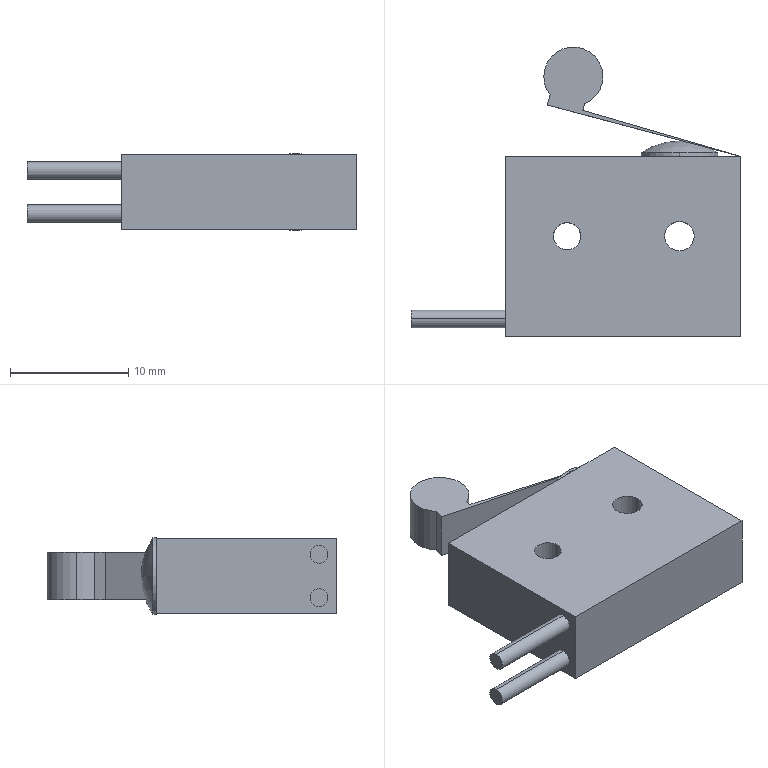Part | SolidWorks | features BaseBody 2 | 2 solids | 32 faces | box 27.9 x 24.5 x 6.5 mm | volume 2034 mm3 | plane 17 | cylinder 13 | sphere 2 | commonest cylinder face diameters 1.5 x4 5 x3 2.3 x2 2.5 x2 6.5 x2
STEP:
#1=CARTESIAN_POINT('',(-1.725,14.375,2.));
#2=VERTEX_POINT('',#1);
#3=CARTESIAN_POINT('',(-6.725,14.375,2.));
#4=VERTEX_POINT('',#3);
#5=CARTESIAN_POINT('',(-4.225,14.375,2.));
#6=DIRECTION('',(0.,0.,1.));
#7=DIRECTION('',(1.,0.,0.));
#8=AXIS2_PLACEMENT_3D('',#5,#6,#7);
#9=CIRCLE('',#8,2.5);
#10=EDGE_CURVE('',#2,#4,#9,.T.);
#11=ORIENTED_EDGE('',*,*,#10,.F.);
#12=CARTESIAN_POINT('',(-1.725,14.375,-2.));
#13=VERTEX_POINT('',#12);
#14=CARTESIAN_POINT('',(-1.725,14.375,2.));
#15=DIRECTION('',(0.,0.,-1.));
#16=VECTOR('',#15,1000.);
#17=LINE('',#14,#16);
#18=EDGE_CURVE('',#2,#13,#17,.T.);
#19=ORIENTED_EDGE('',*,*,#18,.T.);
#20=CARTESIAN_POINT('',(-6.725,14.375,-2.));
#21=VERTEX_POINT('',#20);
#22=CARTESIAN_POINT('',(-4.225,14.375,-2.));
#23=DIRECTION('',(0.,0.,1.));
#24=DIRECTION('',(1.,0.,0.));
#25=AXIS2_PLACEMENT_3D('',#22,#23,#24);
#26=CIRCLE('',#25,2.5);
#27=EDGE_CURVE('',#13,#21,#26,.T.);
#28=ORIENTED_EDGE('',*,*,#27,.T.);
#29=CARTESIAN_POINT('',(-6.725,14.375,2.));
#30=DIRECTION('',(0.,0.,-1.));
#31=VECTOR('',#30,1000.);
#32=LINE('',#29,#31);
#33=EDGE_CURVE('',#4,#21,#32,.T.);
#34=ORIENTED_EDGE('',*,*,#33,.F.);
#35=EDGE_LOOP('',(#11,#19,#28,#34));
#36=FACE_OUTER_BOUND('',#35,.T.);
#37=CARTESIAN_POINT('',(-4.225,14.375,2.));
#38=DIRECTION('',(0.,0.,-1.));
#39=DIRECTION('',(-1.,0.,0.));
#40=AXIS2_PLACEMENT_3D('',#37,#38,#39);
#41=CYLINDRICAL_SURFACE('',#40,2.5);
#42=ADVANCED_FACE('',(#36),#41,.T.);
#43=CARTESIAN_POINT('',(-6.187,12.826,2.));
#44=VERTEX_POINT('',#43);
#45=CARTESIAN_POINT('',(-4.225,14.375,2.));
#46=DIRECTION('',(0.,0.,1.));
#47=DIRECTION('',(1.,0.,0.));
#48=AXIS2_PLACEMENT_3D('',#45,#46,#47);
#49=CIRCLE('',#48,2.5);
#50=EDGE_CURVE('',#4,#44,#49,.T.);
#51=ORIENTED_EDGE('',*,*,#50,.F.);
#52=ORIENTED_EDGE('',*,*,#33,.T.);
#53=CARTESIAN_POINT('',(-6.187,12.826,-2.));
#54=VERTEX_POINT('',#53);
#55=CARTESIAN_POINT('',(-4.225,14.375,-2.));
#56=DIRECTION('',(0.,0.,1.));
#57=DIRECTION('',(1.,0.,0.));
#58=AXIS2_PLACEMENT_3D('',#55,#56,#57);
#59=CIRCLE('',#58,2.5);
#60=EDGE_CURVE('',#21,#54,#59,.T.);
#61=ORIENTED_EDGE('',*,*,#60,.T.);
#62=CARTESIAN_POINT('',(-6.187,12.826,2.));
#63=DIRECTION('',(0.,0.,-1.));
#64=VECTOR('',#63,1000.);
#65=LINE('',#62,#64);
#66=EDGE_CURVE('',#44,#54,#65,.T.);
#67=ORIENTED_EDGE('',*,*,#66,.F.);
#68=EDGE_LOOP('',(#51,#52,#61,#67));
#69=FACE_OUTER_BOUND('',#68,.T.);
#70=CARTESIAN_POINT('',(-4.225,14.375,2.));
#71=DIRECTION('',(0.,0.,-1.));
#72=DIRECTION('',(-1.,0.,0.));
#73=AXIS2_PLACEMENT_3D('',#70,#71,#72);
#74=CYLINDRICAL_SURFACE('',#73,2.5);
#75=ADVANCED_FACE('',(#69),#74,.T.);
#76=CARTESIAN_POINT('',(-3.429,11.526,-2.));
#77=VERTEX_POINT('',#76);
#78=CARTESIAN_POINT('',(9.95,7.625,-2.));
#79=VERTEX_POINT('',#78);
#80=CARTESIAN_POINT('',(-3.429,11.526,-2.));
#81=DIRECTION('',(0.96,-0.2799,0.));
#82=VECTOR('',#81,1000.);
#83=LINE('',#80,#82);
#84=EDGE_CURVE('',#77,#79,#83,.T.);
#85=ORIENTED_EDGE('',*,*,#84,.F.);
#86=CARTESIAN_POINT('',(-3.429,11.526,2.));
#87=VERTEX_POINT('',#86);
#88=CARTESIAN_POINT('',(-3.429,11.526,2.));
#89=DIRECTION('',(0.,0.,-1.));
#90=VECTOR('',#89,1000.);
#91=LINE('',#88,#90);
#92=EDGE_CURVE('',#87,#77,#91,.T.);
#93=ORIENTED_EDGE('',*,*,#92,.F.);
#94=CARTESIAN_POINT('',(9.95,7.625,2.));
#95=VERTEX_POINT('',#94);
#96=CARTESIAN_POINT('',(-3.429,11.526,2.));
#97=DIRECTION('',(0.96,-0.2799,0.));
#98=VECTOR('',#97,1000.);
#99=LINE('',#96,#98);
#100=EDGE_CURVE('',#87,#95,#99,.T.);
#101=ORIENTED_EDGE('',*,*,#100,.T.);
#102=CARTESIAN_POINT('',(9.95,7.625,2.));
#103=DIRECTION('',(0.,0.,-1.));
#104=VECTOR('',#103,1000.);
#105=LINE('',#102,#104);
#106=EDGE_CURVE('',#95,#79,#105,.T.);
#107=ORIENTED_EDGE('',*,*,#106,.T.);
#108=EDGE_LOOP('',(#85,#93,#101,#107));
#109=FACE_OUTER_BOUND('',#108,.T.);
#110=CARTESIAN_POINT('',(-3.429,11.526,2.));
#111=DIRECTION('',(0.2799,0.96,0.));
#112=DIRECTION('',(0.,0.,-1.));
#113=AXIS2_PLACEMENT_3D('',#110,#111,#112);
#114=PLANE('',#113);
#115=ADVANCED_FACE('',(#109),#114,.T.);
#116=CARTESIAN_POINT('',(-3.288,12.057,-2.));
#117=VERTEX_POINT('',#116);
#118=CARTESIAN_POINT('',(-3.288,12.057,-2.));
#119=DIRECTION('',(-0.2564,-0.9666,0.));
#120=VECTOR('',#119,1000.);
#121=LINE('',#118,#120);
#122=EDGE_CURVE('',#117,#77,#121,.T.);
#123=ORIENTED_EDGE('',*,*,#122,.F.);
#124=CARTESIAN_POINT('',(-3.288,12.057,2.));
#125=VERTEX_POINT('',#124);
#126=CARTESIAN_POINT('',(-3.288,12.057,2.));
#127=DIRECTION('',(0.,0.,-1.));
#128=VECTOR('',#127,1000.);
#129=LINE('',#126,#128);
#130=EDGE_CURVE('',#125,#117,#129,.T.);
#131=ORIENTED_EDGE('',*,*,#130,.F.);
#132=CARTESIAN_POINT('',(-3.288,12.057,2.));
#133=DIRECTION('',(-0.2564,-0.9666,0.));
#134=VECTOR('',#133,1000.);
#135=LINE('',#132,#134);
#136=EDGE_CURVE('',#125,#87,#135,.T.);
#137=ORIENTED_EDGE('',*,*,#136,.T.);
#138=ORIENTED_EDGE('',*,*,#92,.T.);
#139=EDGE_LOOP('',(#123,#131,#137,#138));
#140=FACE_OUTER_BOUND('',#139,.T.);
#141=CARTESIAN_POINT('',(-3.288,12.057,2.));
#142=DIRECTION('',(0.9666,-0.2564,0.));
#143=DIRECTION('',(0.,0.,-1.));
#144=AXIS2_PLACEMENT_3D('',#141,#142,#143);
#145=PLANE('',#144);
#146=ADVANCED_FACE('',(#140),#145,.T.);
#147=ORIENTED_EDGE('',*,*,#18,.F.);
#148=CARTESIAN_POINT('',(-4.225,14.375,2.));
#149=DIRECTION('',(0.,0.,1.));
#150=DIRECTION('',(1.,0.,0.));
#151=AXIS2_PLACEMENT_3D('',#148,#149,#150);
#152=CIRCLE('',#151,2.5);
#153=EDGE_CURVE('',#125,#2,#152,.T.);
#154=ORIENTED_EDGE('',*,*,#153,.F.);
#155=ORIENTED_EDGE('',*,*,#130,.T.);
#156=CARTESIAN_POINT('',(-4.225,14.375,-2.));
#157=DIRECTION('',(0.,0.,1.));
#158=DIRECTION('',(1.,0.,0.));
#159=AXIS2_PLACEMENT_3D('',#156,#157,#158);
#160=CIRCLE('',#159,2.5);
#161=EDGE_CURVE('',#117,#13,#160,.T.);
#162=ORIENTED_EDGE('',*,*,#161,.T.);
#163=EDGE_LOOP('',(#147,#154,#155,#162));
#164=FACE_OUTER_BOUND('',#163,.T.);
#165=CARTESIAN_POINT('',(-4.225,14.375,2.));
#166=DIRECTION('',(0.,0.,-1.));
#167=DIRECTION('',(-1.,0.,0.));
#168=AXIS2_PLACEMENT_3D('',#165,#166,#167);
#169=CYLINDRICAL_SURFACE('',#168,2.5);
#170=ADVANCED_FACE('',(#164),#169,.T.);
#171=CARTESIAN_POINT('',(-6.416,11.966,-2.));
#172=VERTEX_POINT('',#171);
#173=CARTESIAN_POINT('',(-6.416,11.966,-2.));
#174=DIRECTION('',(0.2564,0.9666,0.));
#175=VECTOR('',#174,1000.);
#176=LINE('',#173,#175);
#177=EDGE_CURVE('',#172,#54,#176,.T.);
#178=ORIENTED_EDGE('',*,*,#177,.F.);
#179=CARTESIAN_POINT('',(-6.416,11.966,2.));
#180=VERTEX_POINT('',#179);
#181=CARTESIAN_POINT('',(-6.416,11.966,2.));
#182=DIRECTION('',(0.,0.,-1.));
#183=VECTOR('',#182,1000.);
#184=LINE('',#181,#183);
#185=EDGE_CURVE('',#180,#172,#184,.T.);
#186=ORIENTED_EDGE('',*,*,#185,.F.);
#187=CARTESIAN_POINT('',(-6.416,11.966,2.));
#188=DIRECTION('',(0.2564,0.9666,0.));
#189=VECTOR('',#188,1000.);
#190=LINE('',#187,#189);
#191=EDGE_CURVE('',#180,#44,#190,.T.);
#192=ORIENTED_EDGE('',*,*,#191,.T.);
#193=ORIENTED_EDGE('',*,*,#66,.T.);
#194=EDGE_LOOP('',(#178,#186,#192,#193));
#195=FACE_OUTER_BOUND('',#194,.T.);
#196=CARTESIAN_POINT('',(-6.416,11.966,2.));
#197=DIRECTION('',(-0.9666,0.2564,0.));
#198=DIRECTION('',(0.,0.,1.));
#199=AXIS2_PLACEMENT_3D('',#196,#197,#198);
#200=PLANE('',#199);
#201=ADVANCED_FACE('',(#195),#200,.T.);
#202=CARTESIAN_POINT('',(9.95,7.625,-2.));
#203=DIRECTION('',(-0.9666,0.2564,0.));
#204=VECTOR('',#203,1000.);
#205=LINE('',#202,#204);
#206=EDGE_CURVE('',#79,#172,#205,.T.);
#207=ORIENTED_EDGE('',*,*,#206,.F.);
#208=ORIENTED_EDGE('',*,*,#106,.F.);
#209=CARTESIAN_POINT('',(9.95,7.625,2.));
#210=DIRECTION('',(-0.9666,0.2564,0.));
#211=VECTOR('',#210,1000.);
#212=LINE('',#209,#211);
#213=EDGE_CURVE('',#95,#180,#212,.T.);
#214=ORIENTED_EDGE('',*,*,#213,.T.);
#215=ORIENTED_EDGE('',*,*,#185,.T.);
#216=EDGE_LOOP('',(#207,#208,#214,#215));
#217=FACE_OUTER_BOUND('',#216,.T.);
#218=CARTESIAN_POINT('',(9.95,7.625,2.));
#219=DIRECTION('',(-0.2564,-0.9666,0.));
#220=DIRECTION('',(-0.9666,0.2564,0.));
#221=AXIS2_PLACEMENT_3D('',#218,#219,#220);
#222=PLANE('',#221);
#223=ADVANCED_FACE('',(#217),#222,.T.);
#224=ORIENTED_EDGE('',*,*,#100,.F.);
#225=ORIENTED_EDGE('',*,*,#136,.F.);
#226=ORIENTED_EDGE('',*,*,#153,.T.);
#227=ORIENTED_EDGE('',*,*,#10,.T.);
#228=ORIENTED_EDGE('',*,*,#50,.T.);
#229=ORIENTED_EDGE('',*,*,#191,.F.);
#230=ORIENTED_EDGE('',*,*,#213,.F.);
#231=EDGE_LOOP('',(#224,#225,#226,#227,#228,#229,#230));
#232=FACE_OUTER_BOUND('',#231,.T.);
#233=CARTESIAN_POINT('',(-4.225,14.375,2.));
#234=DIRECTION('',(0.,0.,1.));
#235=DIRECTION('',(1.,0.,0.));
#236=AXIS2_PLACEMENT_3D('',#233,#234,#235);
#237=PLANE('',#236);
#238=ADVANCED_FACE('',(#232),#237,.T.);
#239=ORIENTED_EDGE('',*,*,#84,.T.);
#240=ORIENTED_EDGE('',*,*,#206,.T.);
#241=ORIENTED_EDGE('',*,*,#177,.T.);
#242=ORIENTED_EDGE('',*,*,#60,.F.);
#243=ORIENTED_EDGE('',*,*,#27,.F.);
#244=ORIENTED_EDGE('',*,*,#161,.F.);
#245=ORIENTED_EDGE('',*,*,#122,.T.);
#246=EDGE_LOOP('',(#239,#240,#241,#242,#243,#244,#245));
#247=FACE_OUTER_BOUND('',#246,.T.);
#248=CARTESIAN_POINT('',(-4.225,14.375,-2.));
#249=DIRECTION('',(0.,0.,1.));
#250=DIRECTION('',(1.,0.,0.));
#251=AXIS2_PLACEMENT_3D('',#248,#249,#250);
#252=PLANE('',#251);
#253=ADVANCED_FACE('',(#247),#252,.F.);
#254=CLOSED_SHELL('',(#42,#75,#115,#146,#170,#201,#223,#238,#253));
#255=MANIFOLD_SOLID_BREP('',#254);
#256=CARTESIAN_POINT('',(4.75,7.925,-3.25));
#257=VERTEX_POINT('',#256);
#258=CARTESIAN_POINT('',(1.5,7.925,0.));
#259=VERTEX_POINT('',#258);
#260=CARTESIAN_POINT('',(4.75,7.925,0.));
#261=DIRECTION('',(0.,1.,0.));
#262=DIRECTION('',(0.,0.,1.));
#263=AXIS2_PLACEMENT_3D('',#260,#261,#262);
#264=CIRCLE('',#263,3.25);
#265=EDGE_CURVE('',#257,#259,#264,.T.);
#266=ORIENTED_EDGE('',*,*,#265,.T.);
#267=CARTESIAN_POINT('',(4.75,8.925,0.));
#268=VERTEX_POINT('',#267);
#269=CARTESIAN_POINT('',(4.75,3.144,0.));
#270=DIRECTION('',(0.,0.,-1.));
#271=DIRECTION('',(-1.,0.,0.));
#272=AXIS2_PLACEMENT_3D('',#269,#270,#271);
#273=CIRCLE('',#272,5.781);
#274=EDGE_CURVE('',#259,#268,#273,.T.);
#275=ORIENTED_EDGE('',*,*,#274,.T.);
#276=CARTESIAN_POINT('',(8.,7.925,0.));
#277=VERTEX_POINT('',#276);
#278=CARTESIAN_POINT('',(4.75,3.144,0.));
#279=DIRECTION('',(0.,0.,1.));
#280=DIRECTION('',(1.,0.,0.));
#281=AXIS2_PLACEMENT_3D('',#278,#279,#280);
#282=CIRCLE('',#281,5.781);
#283=EDGE_CURVE('',#277,#268,#282,.T.);
#284=ORIENTED_EDGE('',*,*,#283,.F.);
#285=CARTESIAN_POINT('',(4.75,7.925,0.));
#286=DIRECTION('',(0.,1.,0.));
#287=DIRECTION('',(0.,0.,1.));
#288=AXIS2_PLACEMENT_3D('',#285,#286,#287);
#289=CIRCLE('',#288,3.25);
#290=EDGE_CURVE('',#277,#257,#289,.T.);
#291=ORIENTED_EDGE('',*,*,#290,.T.);
#292=EDGE_LOOP('',(#266,#275,#284,#291));
#293=FACE_OUTER_BOUND('',#292,.T.);
#294=CARTESIAN_POINT('',(4.75,3.144,0.));
#295=DIRECTION('',(0.,0.,-1.));
#296=DIRECTION('',(1.,0.,0.));
#297=AXIS2_PLACEMENT_3D('',#294,#295,#296);
#298=SPHERICAL_SURFACE('',#297,5.781);
#299=ADVANCED_FACE('',(#293),#298,.T.);
#300=CARTESIAN_POINT('',(-17.95,-6.125,2.579));
#301=VERTEX_POINT('',#300);
#302=CARTESIAN_POINT('',(-17.95,-6.125,1.079));
#303=VERTEX_POINT('',#302);
#304=CARTESIAN_POINT('',(-17.95,-6.125,1.829));
#305=DIRECTION('',(-1.,0.,0.));
#306=DIRECTION('',(0.,0.,1.));
#307=AXIS2_PLACEMENT_3D('',#304,#305,#306);
#308=CIRCLE('',#307,0.75);
#309=EDGE_CURVE('',#301,#303,#308,.T.);
#310=ORIENTED_EDGE('',*,*,#309,.F.);
#311=CARTESIAN_POINT('',(-9.95,-6.125,2.579));
#312=VERTEX_POINT('',#311);
#313=CARTESIAN_POINT('',(-17.95,-6.125,2.579));
#314=DIRECTION('',(1.,0.,0.));
#315=VECTOR('',#314,1000.);
#316=LINE('',#313,#315);
#317=EDGE_CURVE('',#301,#312,#316,.T.);
#318=ORIENTED_EDGE('',*,*,#317,.T.);
#319=CARTESIAN_POINT('',(-9.95,-6.125,1.079));
#320=VERTEX_POINT('',#319);
#321=CARTESIAN_POINT('',(-9.95,-6.125,1.829));
#322=DIRECTION('',(-1.,0.,0.));
#323=DIRECTION('',(0.,0.,-1.));
#324=AXIS2_PLACEMENT_3D('',#321,#322,#323);
#325=CIRCLE('',#324,0.75);
#326=EDGE_CURVE('',#312,#320,#325,.T.);
#327=ORIENTED_EDGE('',*,*,#326,.T.);
#328=CARTESIAN_POINT('',(-17.95,-6.125,1.079));
#329=DIRECTION('',(1.,0.,0.));
#330=VECTOR('',#329,1000.);
#331=LINE('',#328,#330);
#332=EDGE_CURVE('',#303,#320,#331,.T.);
#333=ORIENTED_EDGE('',*,*,#332,.F.);
#334=EDGE_LOOP('',(#310,#318,#327,#333));
#335=FACE_OUTER_BOUND('',#334,.T.);
#336=CARTESIAN_POINT('',(-17.95,-6.125,1.829));
#337=DIRECTION('',(1.,0.,0.));
#338=DIRECTION('',(0.,0.,-1.));
#339=AXIS2_PLACEMENT_3D('',#336,#337,#338);
#340=CYLINDRICAL_SURFACE('',#339,0.75);
#341=ADVANCED_FACE('',(#335),#340,.T.);
#342=CARTESIAN_POINT('',(-17.95,-6.125,-1.079));
#343=VERTEX_POINT('',#342);
#344=CARTESIAN_POINT('',(-17.95,-6.125,-2.579));
#345=VERTEX_POINT('',#344);
#346=CARTESIAN_POINT('',(-17.95,-6.125,-1.829));
#347=DIRECTION('',(-1.,0.,0.));
#348=DIRECTION('',(0.,0.,1.));
#349=AXIS2_PLACEMENT_3D('',#346,#347,#348);
#350=CIRCLE('',#349,0.75);
#351=EDGE_CURVE('',#343,#345,#350,.T.);
#352=ORIENTED_EDGE('',*,*,#351,.F.);
#353=CARTESIAN_POINT('',(-9.95,-6.125,-1.079));
#354=VERTEX_POINT('',#353);
#355=CARTESIAN_POINT('',(-17.95,-6.125,-1.079));
#356=DIRECTION('',(1.,0.,0.));
#357=VECTOR('',#356,1000.);
#358=LINE('',#355,#357);
#359=EDGE_CURVE('',#343,#354,#358,.T.);
#360=ORIENTED_EDGE('',*,*,#359,.T.);
#361=CARTESIAN_POINT('',(-9.95,-6.125,-2.579));
#362=VERTEX_POINT('',#361);
#363=CARTESIAN_POINT('',(-9.95,-6.125,-1.829));
#364=DIRECTION('',(-1.,0.,0.));
#365=DIRECTION('',(0.,0.,-1.));
#366=AXIS2_PLACEMENT_3D('',#363,#364,#365);
#367=CIRCLE('',#366,0.75);
#368=EDGE_CURVE('',#354,#362,#367,.T.);
#369=ORIENTED_EDGE('',*,*,#368,.T.);
#370=CARTESIAN_POINT('',(-17.95,-6.125,-2.579));
#371=DIRECTION('',(1.,0.,0.));
#372=VECTOR('',#371,1000.);
#373=LINE('',#370,#372);
#374=EDGE_CURVE('',#345,#362,#373,.T.);
#375=ORIENTED_EDGE('',*,*,#374,.F.);
#376=EDGE_LOOP('',(#352,#360,#369,#375));
#377=FACE_OUTER_BOUND('',#376,.T.);
#378=CARTESIAN_POINT('',(-17.95,-6.125,-1.829));
#379=DIRECTION('',(1.,0.,0.));
#380=DIRECTION('',(0.,0.,-1.));
#381=AXIS2_PLACEMENT_3D('',#378,#379,#380);
#382=CYLINDRICAL_SURFACE('',#381,0.75);
#383=ADVANCED_FACE('',(#377),#382,.T.);
#384=CARTESIAN_POINT('',(4.75,7.925,3.25));
#385=VERTEX_POINT('',#384);
#386=CARTESIAN_POINT('',(4.75,7.925,0.));
#387=DIRECTION('',(0.,1.,0.));
#388=DIRECTION('',(0.,0.,1.));
#389=AXIS2_PLACEMENT_3D('',#386,#387,#388);
#390=CIRCLE('',#389,3.25);
#391=EDGE_CURVE('',#385,#277,#390,.T.);
#392=ORIENTED_EDGE('',*,*,#391,.F.);
#393=CARTESIAN_POINT('',(4.75,7.625,3.25));
#394=VERTEX_POINT('',#393);
#395=CARTESIAN_POINT('',(4.75,7.925,3.25));
#396=DIRECTION('',(0.,-1.,0.));
#397=VECTOR('',#396,1000.);
#398=LINE('',#395,#397);
#399=EDGE_CURVE('',#385,#394,#398,.T.);
#400=ORIENTED_EDGE('',*,*,#399,.T.);
#401=CARTESIAN_POINT('',(5.318,7.625,3.2));
#402=VERTEX_POINT('',#401);
#403=CARTESIAN_POINT('',(4.75,7.625,0.));
#404=DIRECTION('',(0.,1.,0.));
#405=DIRECTION('',(0.,0.,1.));
#406=AXIS2_PLACEMENT_3D('',#403,#404,#405);
#407=CIRCLE('',#406,3.25);
#408=EDGE_CURVE('',#394,#402,#407,.T.);
#409=ORIENTED_EDGE('',*,*,#408,.T.);
#410=CARTESIAN_POINT('',(5.318,7.625,-3.2));
#411=VERTEX_POINT('',#410);
#412=CARTESIAN_POINT('',(4.75,7.625,0.));
#413=DIRECTION('',(0.,1.,0.));
#414=DIRECTION('',(0.,0.,1.));
#415=AXIS2_PLACEMENT_3D('',#412,#413,#414);
#416=CIRCLE('',#415,3.25);
#417=EDGE_CURVE('',#402,#411,#416,.T.);
#418=ORIENTED_EDGE('',*,*,#417,.T.);
#419=CARTESIAN_POINT('',(4.75,7.625,-3.25));
#420=VERTEX_POINT('',#419);
#421=CARTESIAN_POINT('',(4.75,7.625,0.));
#422=DIRECTION('',(0.,1.,0.));
#423=DIRECTION('',(0.,0.,1.));
#424=AXIS2_PLACEMENT_3D('',#421,#422,#423);
#425=CIRCLE('',#424,3.25);
#426=EDGE_CURVE('',#411,#420,#425,.T.);
#427=ORIENTED_EDGE('',*,*,#426,.T.);
#428=CARTESIAN_POINT('',(4.75,7.925,-3.25));
#429=DIRECTION('',(0.,-1.,0.));
#430=VECTOR('',#429,1000.);
#431=LINE('',#428,#430);
#432=EDGE_CURVE('',#257,#420,#431,.T.);
#433=ORIENTED_EDGE('',*,*,#432,.F.);
#434=ORIENTED_EDGE('',*,*,#290,.F.);
#435=EDGE_LOOP('',(#392,#400,#409,#418,#427,#433,#434));
#436=FACE_OUTER_BOUND('',#435,.T.);
#437=CARTESIAN_POINT('',(4.75,7.925,0.));
#438=DIRECTION('',(0.,-1.,0.));
#439=DIRECTION('',(0.,0.,-1.));
#440=AXIS2_PLACEMENT_3D('',#437,#438,#439);
#441=CYLINDRICAL_SURFACE('',#440,3.25);
#442=ADVANCED_FACE('',(#436),#441,.T.);
#443=CARTESIAN_POINT('',(3.5,0.875,3.2));
#444=VERTEX_POINT('',#443);
#445=CARTESIAN_POINT('',(6.,0.875,3.2));
#446=VERTEX_POINT('',#445);
#447=CARTESIAN_POINT('',(4.75,0.875,3.2));
#448=DIRECTION('',(0.,0.,1.));
#449=DIRECTION('',(1.,0.,0.));
#450=AXIS2_PLACEMENT_3D('',#447,#448,#449);
#451=CIRCLE('',#450,1.25);
#452=EDGE_CURVE('',#444,#446,#451,.T.);
#453=ORIENTED_EDGE('',*,*,#452,.T.);
#454=CARTESIAN_POINT('',(6.,0.875,-3.2));
#455=VERTEX_POINT('',#454);
#456=CARTESIAN_POINT('',(6.,0.875,3.2));
#457=DIRECTION('',(0.,0.,-1.));
#458=VECTOR('',#457,1000.);
#459=LINE('',#456,#458);
#460=EDGE_CURVE('',#446,#455,#459,.T.);
#461=ORIENTED_EDGE('',*,*,#460,.T.);
#462=CARTESIAN_POINT('',(3.5,0.875,-3.2));
#463=VERTEX_POINT('',#462);
#464=CARTESIAN_POINT('',(4.75,0.875,-3.2));
#465=DIRECTION('',(0.,0.,1.));
#466=DIRECTION('',(1.,0.,0.));
#467=AXIS2_PLACEMENT_3D('',#464,#465,#466);
#468=CIRCLE('',#467,1.25);
#469=EDGE_CURVE('',#463,#455,#468,.T.);
#470=ORIENTED_EDGE('',*,*,#469,.F.);
#471=CARTESIAN_POINT('',(3.5,0.875,3.2));
#472=DIRECTION('',(0.,0.,-1.));
#473=VECTOR('',#472,1000.);
#474=LINE('',#471,#473);
#475=EDGE_CURVE('',#444,#463,#474,.T.);
#476=ORIENTED_EDGE('',*,*,#475,.F.);
#477=EDGE_LOOP('',(#453,#461,#470,#476));
#478=FACE_OUTER_BOUND('',#477,.T.);
#479=CARTESIAN_POINT('',(4.75,0.875,3.2));
#480=DIRECTION('',(0.,0.,-1.));
#481=DIRECTION('',(-1.,0.,0.));
#482=AXIS2_PLACEMENT_3D('',#479,#480,#481);
#483=CYLINDRICAL_SURFACE('',#482,1.25);
#484=ADVANCED_FACE('',(#478),#483,.F.);
#485=CARTESIAN_POINT('',(-5.9,0.875,3.2));
#486=VERTEX_POINT('',#485);
#487=CARTESIAN_POINT('',(-3.6,0.875,3.2));
#488=VERTEX_POINT('',#487);
#489=CARTESIAN_POINT('',(-4.75,0.875,3.2));
#490=DIRECTION('',(0.,0.,1.));
#491=DIRECTION('',(1.,0.,0.));
#492=AXIS2_PLACEMENT_3D('',#489,#490,#491);
#493=CIRCLE('',#492,1.15);
#494=EDGE_CURVE('',#486,#488,#493,.T.);
#495=ORIENTED_EDGE('',*,*,#494,.T.);
#496=CARTESIAN_POINT('',(-3.6,0.875,-3.2));
#497=VERTEX_POINT('',#496);
#498=CARTESIAN_POINT('',(-3.6,0.875,3.2));
#499=DIRECTION('',(0.,0.,-1.));
#500=VECTOR('',#499,1000.);
#501=LINE('',#498,#500);
#502=EDGE_CURVE('',#488,#497,#501,.T.);
#503=ORIENTED_EDGE('',*,*,#502,.T.);
#504=CARTESIAN_POINT('',(-5.9,0.875,-3.2));
#505=VERTEX_POINT('',#504);
#506=CARTESIAN_POINT('',(-4.75,0.875,-3.2));
#507=DIRECTION('',(0.,0.,1.));
#508=DIRECTION('',(1.,0.,0.));
#509=AXIS2_PLACEMENT_3D('',#506,#507,#508);
#510=CIRCLE('',#509,1.15);
#511=EDGE_CURVE('',#505,#497,#510,.T.);
#512=ORIENTED_EDGE('',*,*,#511,.F.);
#513=CARTESIAN_POINT('',(-5.9,0.875,3.2));
#514=DIRECTION('',(0.,0.,-1.));
#515=VECTOR('',#514,1000.);
#516=LINE('',#513,#515);
#517=EDGE_CURVE('',#486,#505,#516,.T.);
#518=ORIENTED_EDGE('',*,*,#517,.F.);
#519=EDGE_LOOP('',(#495,#503,#512,#518));
#520=FACE_OUTER_BOUND('',#519,.T.);
#521=CARTESIAN_POINT('',(-4.75,0.875,3.2));
#522=DIRECTION('',(0.,0.,-1.));
#523=DIRECTION('',(-1.,0.,0.));
#524=AXIS2_PLACEMENT_3D('',#521,#522,#523);
#525=CYLINDRICAL_SURFACE('',#524,1.15);
#526=ADVANCED_FACE('',(#520),#525,.F.);
#527=ORIENTED_EDGE('',*,*,#417,.F.);
#528=CARTESIAN_POINT('',(9.95,7.625,3.2));
#529=VERTEX_POINT('',#528);
#530=CARTESIAN_POINT('',(-9.95,7.625,3.2));
#531=DIRECTION('',(-1.,0.,0.));
#532=VECTOR('',#531,1000.);
#533=LINE('',#530,#532);
#534=EDGE_CURVE('',#529,#402,#533,.T.);
#535=ORIENTED_EDGE('',*,*,#534,.F.);
#536=CARTESIAN_POINT('',(9.95,7.625,-3.2));
#537=VERTEX_POINT('',#536);
#538=CARTESIAN_POINT('',(9.95,7.625,3.2));
#539=DIRECTION('',(0.,0.,-1.));
#540=VECTOR('',#539,1000.);
#541=LINE('',#538,#540);
#542=EDGE_CURVE('',#529,#537,#541,.T.);
#543=ORIENTED_EDGE('',*,*,#542,.T.);
#544=CARTESIAN_POINT('',(-9.95,7.625,-3.2));
#545=DIRECTION('',(-1.,0.,0.));
#546=VECTOR('',#545,1000.);
#547=LINE('',#544,#546);
#548=EDGE_CURVE('',#537,#411,#547,.T.);
#549=ORIENTED_EDGE('',*,*,#548,.T.);
#550=EDGE_LOOP('',(#527,#535,#543,#549));
#551=FACE_OUTER_BOUND('',#550,.T.);
#552=CARTESIAN_POINT('',(-9.95,7.625,3.2));
#553=DIRECTION('',(0.,-1.,0.));
#554=DIRECTION('',(0.,0.,-1.));
#555=AXIS2_PLACEMENT_3D('',#552,#553,#554);
#556=PLANE('',#555);
#557=ADVANCED_FACE('',(#551),#556,.F.);
#558=CARTESIAN_POINT('',(9.95,-7.625,3.2));
#559=VERTEX_POINT('',#558);
#560=CARTESIAN_POINT('',(9.95,7.625,3.2));
#561=DIRECTION('',(0.,1.,0.));
#562=VECTOR('',#561,1000.);
#563=LINE('',#560,#562);
#564=EDGE_CURVE('',#559,#529,#563,.T.);
#565=ORIENTED_EDGE('',*,*,#564,.T.);
#566=ORIENTED_EDGE('',*,*,#534,.T.);
#567=CARTESIAN_POINT('',(4.182,7.625,3.2));
#568=VERTEX_POINT('',#567);
#569=CARTESIAN_POINT('',(-9.95,7.625,3.2));
#570=DIRECTION('',(-1.,0.,0.));
#571=VECTOR('',#570,1000.);
#572=LINE('',#569,#571);
#573=EDGE_CURVE('',#402,#568,#572,.T.);
#574=ORIENTED_EDGE('',*,*,#573,.T.);
#575=CARTESIAN_POINT('',(-9.95,7.625,3.2));
#576=VERTEX_POINT('',#575);
#577=CARTESIAN_POINT('',(-9.95,7.625,3.2));
#578=DIRECTION('',(-1.,0.,0.));
#579=VECTOR('',#578,1000.);
#580=LINE('',#577,#579);
#581=EDGE_CURVE('',#568,#576,#580,.T.);
#582=ORIENTED_EDGE('',*,*,#581,.T.);
#583=CARTESIAN_POINT('',(-9.95,-7.625,3.2));
#584=VERTEX_POINT('',#583);
#585=CARTESIAN_POINT('',(-9.95,7.625,3.2));
#586=DIRECTION('',(0.,-1.,0.));
#587=VECTOR('',#586,1000.);
#588=LINE('',#585,#587);
#589=EDGE_CURVE('',#576,#584,#588,.T.);
#590=ORIENTED_EDGE('',*,*,#589,.T.);
#591=CARTESIAN_POINT('',(-9.95,-7.625,3.2));
#592=DIRECTION('',(1.,0.,0.));
#593=VECTOR('',#592,1000.);
#594=LINE('',#591,#593);
#595=EDGE_CURVE('',#584,#559,#594,.T.);
#596=ORIENTED_EDGE('',*,*,#595,.T.);
#597=EDGE_LOOP('',(#565,#566,#574,#582,#590,#596));
#598=FACE_OUTER_BOUND('',#597,.T.);
#599=ORIENTED_EDGE('',*,*,#494,.F.);
#600=CARTESIAN_POINT('',(-4.75,0.875,3.2));
#601=DIRECTION('',(0.,0.,1.));
#602=DIRECTION('',(1.,0.,0.));
#603=AXIS2_PLACEMENT_3D('',#600,#601,#602);
#604=CIRCLE('',#603,1.15);
#605=EDGE_CURVE('',#488,#486,#604,.T.);
#606=ORIENTED_EDGE('',*,*,#605,.F.);
#607=EDGE_LOOP('',(#599,#606));
#608=FACE_BOUND('',#607,.T.);
#609=ORIENTED_EDGE('',*,*,#452,.F.);
#610=CARTESIAN_POINT('',(4.75,0.875,3.2));
#611=DIRECTION('',(0.,0.,1.));
#612=DIRECTION('',(1.,0.,0.));
#613=AXIS2_PLACEMENT_3D('',#610,#611,#612);
#614=CIRCLE('',#613,1.25);
#615=EDGE_CURVE('',#446,#444,#614,.T.);
#616=ORIENTED_EDGE('',*,*,#615,.F.);
#617=EDGE_LOOP('',(#609,#616));
#618=FACE_BOUND('',#617,.T.);
#619=CARTESIAN_POINT('',(0.,0.,3.2));
#620=DIRECTION('',(0.,0.,1.));
#621=DIRECTION('',(1.,0.,0.));
#622=AXIS2_PLACEMENT_3D('',#619,#620,#621);
#623=PLANE('',#622);
#624=ADVANCED_FACE('',(#598,#608,#618),#623,.T.);
#625=CARTESIAN_POINT('',(9.95,-7.625,-3.2));
#626=VERTEX_POINT('',#625);
#627=CARTESIAN_POINT('',(9.95,7.625,-3.2));
#628=DIRECTION('',(0.,1.,0.));
#629=VECTOR('',#628,1000.);
#630=LINE('',#627,#629);
#631=EDGE_CURVE('',#626,#537,#630,.T.);
#632=ORIENTED_EDGE('',*,*,#631,.F.);
#633=CARTESIAN_POINT('',(-9.95,-7.625,-3.2));
#634=VERTEX_POINT('',#633);
#635=CARTESIAN_POINT('',(-9.95,-7.625,-3.2));
#636=DIRECTION('',(1.,0.,0.));
#637=VECTOR('',#636,1000.);
#638=LINE('',#635,#637);
#639=EDGE_CURVE('',#634,#626,#638,.T.);
#640=ORIENTED_EDGE('',*,*,#639,.F.);
#641=CARTESIAN_POINT('',(-9.95,7.625,-3.2));
#642=VERTEX_POINT('',#641);
#643=CARTESIAN_POINT('',(-9.95,7.625,-3.2));
#644=DIRECTION('',(0.,-1.,0.));
#645=VECTOR('',#644,1000.);
#646=LINE('',#643,#645);
#647=EDGE_CURVE('',#642,#634,#646,.T.);
#648=ORIENTED_EDGE('',*,*,#647,.F.);
#649=CARTESIAN_POINT('',(4.182,7.625,-3.2));
#650=VERTEX_POINT('',#649);
#651=CARTESIAN_POINT('',(-9.95,7.625,-3.2));
#652=DIRECTION('',(-1.,0.,0.));
#653=VECTOR('',#652,1000.);
#654=LINE('',#651,#653);
#655=EDGE_CURVE('',#650,#642,#654,.T.);
#656=ORIENTED_EDGE('',*,*,#655,.F.);
#657=CARTESIAN_POINT('',(-9.95,7.625,-3.2));
#658=DIRECTION('',(-1.,0.,0.));
#659=VECTOR('',#658,1000.);
#660=LINE('',#657,#659);
#661=EDGE_CURVE('',#411,#650,#660,.T.);
#662=ORIENTED_EDGE('',*,*,#661,.F.);
#663=ORIENTED_EDGE('',*,*,#548,.F.);
#664=EDGE_LOOP('',(#632,#640,#648,#656,#662,#663));
#665=FACE_OUTER_BOUND('',#664,.T.);
#666=ORIENTED_EDGE('',*,*,#511,.T.);
#667=CARTESIAN_POINT('',(-4.75,0.875,-3.2));
#668=DIRECTION('',(0.,0.,1.));
#669=DIRECTION('',(1.,0.,0.));
#670=AXIS2_PLACEMENT_3D('',#667,#668,#669);
#671=CIRCLE('',#670,1.15);
#672=EDGE_CURVE('',#497,#505,#671,.T.);
#673=ORIENTED_EDGE('',*,*,#672,.T.);
#674=EDGE_LOOP('',(#666,#673));
#675=FACE_BOUND('',#674,.T.);
#676=ORIENTED_EDGE('',*,*,#469,.T.);
#677=CARTESIAN_POINT('',(4.75,0.875,-3.2));
#678=DIRECTION('',(0.,0.,1.));
#679=DIRECTION('',(1.,0.,0.));
#680=AXIS2_PLACEMENT_3D('',#677,#678,#679);
#681=CIRCLE('',#680,1.25);
#682=EDGE_CURVE('',#455,#463,#681,.T.);
#683=ORIENTED_EDGE('',*,*,#682,.T.);
#684=EDGE_LOOP('',(#676,#683));
#685=FACE_BOUND('',#684,.T.);
#686=CARTESIAN_POINT('',(0.,0.,-3.2));
#687=DIRECTION('',(0.,0.,1.));
#688=DIRECTION('',(1.,0.,0.));
#689=AXIS2_PLACEMENT_3D('',#686,#687,#688);
#690=PLANE('',#689);
#691=ADVANCED_FACE('',(#665,#675,#685),#690,.F.);
#692=ORIENTED_EDGE('',*,*,#631,.T.);
#693=ORIENTED_EDGE('',*,*,#542,.F.);
#694=ORIENTED_EDGE('',*,*,#564,.F.);
#695=CARTESIAN_POINT('',(9.95,-7.625,3.2));
#696=DIRECTION('',(0.,0.,-1.));
#697=VECTOR('',#696,1000.);
#698=LINE('',#695,#697);
#699=EDGE_CURVE('',#559,#626,#698,.T.);
#700=ORIENTED_EDGE('',*,*,#699,.T.);
#701=EDGE_LOOP('',(#692,#693,#694,#700));
#702=FACE_OUTER_BOUND('',#701,.T.);
#703=CARTESIAN_POINT('',(9.95,7.625,3.2));
#704=DIRECTION('',(-1.,0.,0.));
#705=DIRECTION('',(0.,0.,1.));
#706=AXIS2_PLACEMENT_3D('',#703,#704,#705);
#707=PLANE('',#706);
#708=ADVANCED_FACE('',(#702),#707,.F.);
#709=CARTESIAN_POINT('',(4.75,7.625,0.));
#710=DIRECTION('',(0.,1.,0.));
#711=DIRECTION('',(0.,0.,1.));
#712=AXIS2_PLACEMENT_3D('',#709,#710,#711);
#713=CIRCLE('',#712,3.25);
#714=EDGE_CURVE('',#650,#568,#713,.T.);
#715=ORIENTED_EDGE('',*,*,#714,.F.);
#716=ORIENTED_EDGE('',*,*,#655,.T.);
#717=CARTESIAN_POINT('',(-9.95,7.625,3.2));
#718=DIRECTION('',(0.,0.,-1.));
#719=VECTOR('',#718,1000.);
#720=LINE('',#717,#719);
#721=EDGE_CURVE('',#576,#642,#720,.T.);
#722=ORIENTED_EDGE('',*,*,#721,.F.);
#723=ORIENTED_EDGE('',*,*,#581,.F.);
#724=EDGE_LOOP('',(#715,#716,#722,#723));
#725=FACE_OUTER_BOUND('',#724,.T.);
#726=CARTESIAN_POINT('',(-9.95,7.625,3.2));
#727=DIRECTION('',(0.,-1.,0.));
#728=DIRECTION('',(0.,0.,-1.));
#729=AXIS2_PLACEMENT_3D('',#726,#727,#728);
#730=PLANE('',#729);
#731=ADVANCED_FACE('',(#725),#730,.F.);
#732=ORIENTED_EDGE('',*,*,#647,.T.);
#733=CARTESIAN_POINT('',(-9.95,-7.625,3.2));
#734=DIRECTION('',(0.,0.,-1.));
#735=VECTOR('',#734,1000.);
#736=LINE('',#733,#735);
#737=EDGE_CURVE('',#584,#634,#736,.T.);
#738=ORIENTED_EDGE('',*,*,#737,.F.);
#739=ORIENTED_EDGE('',*,*,#589,.F.);
#740=ORIENTED_EDGE('',*,*,#721,.T.);
#741=EDGE_LOOP('',(#732,#738,#739,#740));
#742=FACE_OUTER_BOUND('',#741,.T.);
#743=CARTESIAN_POINT('',(-9.95,-6.125,1.829));
#744=DIRECTION('',(-1.,0.,0.));
#745=DIRECTION('',(0.,0.,-1.));
#746=AXIS2_PLACEMENT_3D('',#743,#744,#745);
#747=CIRCLE('',#746,0.75);
#748=EDGE_CURVE('',#320,#312,#747,.T.);
#749=ORIENTED_EDGE('',*,*,#748,.F.);
#750=ORIENTED_EDGE('',*,*,#326,.F.);
#751=EDGE_LOOP('',(#749,#750));
#752=FACE_BOUND('',#751,.T.);
#753=CARTESIAN_POINT('',(-9.95,-6.125,-1.829));
#754=DIRECTION('',(-1.,0.,0.));
#755=DIRECTION('',(0.,0.,-1.));
#756=AXIS2_PLACEMENT_3D('',#753,#754,#755);
#757=CIRCLE('',#756,0.75);
#758=EDGE_CURVE('',#362,#354,#757,.T.);
#759=ORIENTED_EDGE('',*,*,#758,.F.);
#760=ORIENTED_EDGE('',*,*,#368,.F.);
#761=EDGE_LOOP('',(#759,#760));
#762=FACE_BOUND('',#761,.T.);
#763=CARTESIAN_POINT('',(-9.95,7.625,3.2));
#764=DIRECTION('',(1.,0.,0.));
#765=DIRECTION('',(0.,1.,0.));
#766=AXIS2_PLACEMENT_3D('',#763,#764,#765);
#767=PLANE('',#766);
#768=ADVANCED_FACE('',(#742,#752,#762),#767,.F.);
#769=ORIENTED_EDGE('',*,*,#639,.T.);
#770=ORIENTED_EDGE('',*,*,#699,.F.);
#771=ORIENTED_EDGE('',*,*,#595,.F.);
#772=ORIENTED_EDGE('',*,*,#737,.T.);
#773=EDGE_LOOP('',(#769,#770,#771,#772));
#774=FACE_OUTER_BOUND('',#773,.T.);
#775=CARTESIAN_POINT('',(-9.95,-7.625,3.2));
#776=DIRECTION('',(0.,1.,0.));
#777=DIRECTION('',(1.,0.,0.));
#778=AXIS2_PLACEMENT_3D('',#775,#776,#777);
#779=PLANE('',#778);
#780=ADVANCED_FACE('',(#774),#779,.F.);
#781=ORIENTED_EDGE('',*,*,#502,.F.);
#782=ORIENTED_EDGE('',*,*,#605,.T.);
#783=ORIENTED_EDGE('',*,*,#517,.T.);
#784=ORIENTED_EDGE('',*,*,#672,.F.);
#785=EDGE_LOOP('',(#781,#782,#783,#784));
#786=FACE_OUTER_BOUND('',#785,.T.);
#787=CARTESIAN_POINT('',(-4.75,0.875,3.2));
#788=DIRECTION('',(0.,0.,-1.));
#789=DIRECTION('',(-1.,0.,0.));
#790=AXIS2_PLACEMENT_3D('',#787,#788,#789);
#791=CYLINDRICAL_SURFACE('',#790,1.15);
#792=ADVANCED_FACE('',(#786),#791,.F.);
#793=ORIENTED_EDGE('',*,*,#460,.F.);
#794=ORIENTED_EDGE('',*,*,#615,.T.);
#795=ORIENTED_EDGE('',*,*,#475,.T.);
#796=ORIENTED_EDGE('',*,*,#682,.F.);
#797=EDGE_LOOP('',(#793,#794,#795,#796));
#798=FACE_OUTER_BOUND('',#797,.T.);
#799=CARTESIAN_POINT('',(4.75,0.875,3.2));
#800=DIRECTION('',(0.,0.,-1.));
#801=DIRECTION('',(-1.,0.,0.));
#802=AXIS2_PLACEMENT_3D('',#799,#800,#801);
#803=CYLINDRICAL_SURFACE('',#802,1.25);
#804=ADVANCED_FACE('',(#798),#803,.F.);
#805=ORIENTED_EDGE('',*,*,#426,.F.);
#806=ORIENTED_EDGE('',*,*,#661,.T.);
#807=CARTESIAN_POINT('',(4.75,7.625,0.));
#808=DIRECTION('',(0.,1.,0.));
#809=DIRECTION('',(0.,0.,1.));
#810=AXIS2_PLACEMENT_3D('',#807,#808,#809);
#811=CIRCLE('',#810,3.25);
#812=EDGE_CURVE('',#420,#650,#811,.T.);
#813=ORIENTED_EDGE('',*,*,#812,.F.);
#814=EDGE_LOOP('',(#805,#806,#813));
#815=FACE_OUTER_BOUND('',#814,.T.);
#816=CARTESIAN_POINT('',(4.75,7.625,0.));
#817=DIRECTION('',(0.,1.,0.));
#818=DIRECTION('',(1.,0.,0.));
#819=AXIS2_PLACEMENT_3D('',#816,#817,#818);
#820=PLANE('',#819);
#821=ADVANCED_FACE('',(#815),#820,.F.);
#822=ORIENTED_EDGE('',*,*,#399,.F.);
#823=CARTESIAN_POINT('',(4.75,7.925,0.));
#824=DIRECTION('',(0.,1.,0.));
#825=DIRECTION('',(0.,0.,1.));
#826=AXIS2_PLACEMENT_3D('',#823,#824,#825);
#827=CIRCLE('',#826,3.25);
#828=EDGE_CURVE('',#259,#385,#827,.T.);
#829=ORIENTED_EDGE('',*,*,#828,.F.);
#830=ORIENTED_EDGE('',*,*,#265,.F.);
#831=ORIENTED_EDGE('',*,*,#432,.T.);
#832=ORIENTED_EDGE('',*,*,#812,.T.);
#833=ORIENTED_EDGE('',*,*,#714,.T.);
#834=CARTESIAN_POINT('',(4.75,7.625,0.));
#835=DIRECTION('',(0.,1.,0.));
#836=DIRECTION('',(0.,0.,1.));
#837=AXIS2_PLACEMENT_3D('',#834,#835,#836);
#838=CIRCLE('',#837,3.25);
#839=EDGE_CURVE('',#568,#394,#838,.T.);
#840=ORIENTED_EDGE('',*,*,#839,.T.);
#841=EDGE_LOOP('',(#822,#829,#830,#831,#832,#833,#840));
#842=FACE_OUTER_BOUND('',#841,.T.);
#843=CARTESIAN_POINT('',(4.75,7.925,0.));
#844=DIRECTION('',(0.,-1.,0.));
#845=DIRECTION('',(0.,0.,-1.));
#846=AXIS2_PLACEMENT_3D('',#843,#844,#845);
#847=CYLINDRICAL_SURFACE('',#846,3.25);
#848=ADVANCED_FACE('',(#842),#847,.T.);
#849=ORIENTED_EDGE('',*,*,#274,.F.);
#850=ORIENTED_EDGE('',*,*,#828,.T.);
#851=ORIENTED_EDGE('',*,*,#391,.T.);
#852=ORIENTED_EDGE('',*,*,#283,.T.);
#853=EDGE_LOOP('',(#849,#850,#851,#852));
#854=FACE_OUTER_BOUND('',#853,.T.);
#855=CARTESIAN_POINT('',(4.75,3.144,0.));
#856=DIRECTION('',(0.,0.,-1.));
#857=DIRECTION('',(1.,0.,0.));
#858=AXIS2_PLACEMENT_3D('',#855,#856,#857);
#859=SPHERICAL_SURFACE('',#858,5.781);
#860=ADVANCED_FACE('',(#854),#859,.T.);
#861=ORIENTED_EDGE('',*,*,#573,.F.);
#862=ORIENTED_EDGE('',*,*,#408,.F.);
#863=ORIENTED_EDGE('',*,*,#839,.F.);
#864=EDGE_LOOP('',(#861,#862,#863));
#865=FACE_OUTER_BOUND('',#864,.T.);
#866=CARTESIAN_POINT('',(4.75,7.625,0.));
#867=DIRECTION('',(0.,1.,0.));
#868=DIRECTION('',(1.,0.,0.));
#869=AXIS2_PLACEMENT_3D('',#866,#867,#868);
#870=PLANE('',#869);
#871=ADVANCED_FACE('',(#865),#870,.F.);
#872=ORIENTED_EDGE('',*,*,#359,.F.);
#873=CARTESIAN_POINT('',(-17.95,-6.125,-1.829));
#874=DIRECTION('',(-1.,0.,0.));
#875=DIRECTION('',(0.,0.,1.));
#876=AXIS2_PLACEMENT_3D('',#873,#874,#875);
#877=CIRCLE('',#876,0.75);
#878=EDGE_CURVE('',#345,#343,#877,.T.);
#879=ORIENTED_EDGE('',*,*,#878,.F.);
#880=ORIENTED_EDGE('',*,*,#374,.T.);
#881=ORIENTED_EDGE('',*,*,#758,.T.);
#882=EDGE_LOOP('',(#872,#879,#880,#881));
#883=FACE_OUTER_BOUND('',#882,.T.);
#884=CARTESIAN_POINT('',(-17.95,-6.125,-1.829));
#885=DIRECTION('',(1.,0.,0.));
#886=DIRECTION('',(0.,0.,-1.));
#887=AXIS2_PLACEMENT_3D('',#884,#885,#886);
#888=CYLINDRICAL_SURFACE('',#887,0.75);
#889=ADVANCED_FACE('',(#883),#888,.T.);
#890=ORIENTED_EDGE('',*,*,#878,.T.);
#891=ORIENTED_EDGE('',*,*,#351,.T.);
#892=EDGE_LOOP('',(#890,#891));
#893=FACE_OUTER_BOUND('',#892,.T.);
#894=CARTESIAN_POINT('',(-17.95,-6.125,-1.829));
#895=DIRECTION('',(-1.,0.,0.));
#896=DIRECTION('',(0.,0.,1.));
#897=AXIS2_PLACEMENT_3D('',#894,#895,#896);
#898=PLANE('',#897);
#899=ADVANCED_FACE('',(#893),#898,.T.);
#900=ORIENTED_EDGE('',*,*,#317,.F.);
#901=CARTESIAN_POINT('',(-17.95,-6.125,1.829));
#902=DIRECTION('',(-1.,0.,0.));
#903=DIRECTION('',(0.,0.,1.));
#904=AXIS2_PLACEMENT_3D('',#901,#902,#903);
#905=CIRCLE('',#904,0.75);
#906=EDGE_CURVE('',#303,#301,#905,.T.);
#907=ORIENTED_EDGE('',*,*,#906,.F.);
#908=ORIENTED_EDGE('',*,*,#332,.T.);
#909=ORIENTED_EDGE('',*,*,#748,.T.);
#910=EDGE_LOOP('',(#900,#907,#908,#909));
#911=FACE_OUTER_BOUND('',#910,.T.);
#912=CARTESIAN_POINT('',(-17.95,-6.125,1.829));
#913=DIRECTION('',(1.,0.,0.));
#914=DIRECTION('',(0.,0.,-1.));
#915=AXIS2_PLACEMENT_3D('',#912,#913,#914);
#916=CYLINDRICAL_SURFACE('',#915,0.75);
#917=ADVANCED_FACE('',(#911),#916,.T.);
#918=ORIENTED_EDGE('',*,*,#906,.T.);
#919=ORIENTED_EDGE('',*,*,#309,.T.);
#920=EDGE_LOOP('',(#918,#919));
#921=FACE_OUTER_BOUND('',#920,.T.);
#922=CARTESIAN_POINT('',(-17.95,-6.125,1.829));
#923=DIRECTION('',(-1.,0.,0.));
#924=DIRECTION('',(0.,0.,1.));
#925=AXIS2_PLACEMENT_3D('',#922,#923,#924);
#926=PLANE('',#925);
#927=ADVANCED_FACE('',(#921),#926,.T.);
#928=CLOSED_SHELL('',(#299,#341,#383,#442,#484,#526,#557,#624,#691,#708,#731,#768,#780,#792,#804,#821,#848,#860,#871,#889,#899,#917,#927));
#929=MANIFOLD_SOLID_BREP('',#928);
#930=CARTESIAN_POINT('',(0.,0.,0.));
#931=DIRECTION('',(0.,0.,1.));
#932=DIRECTION('',(1.,0.,0.));
#933=AXIS2_PLACEMENT_3D('',#930,#931,#932);
#934=(LENGTH_UNIT()NAMED_UNIT(*)SI_UNIT(.MILLI.,.METRE.));
#935=UNCERTAINTY_MEASURE_WITH_UNIT(LENGTH_MEASURE(0.00001),#934,'','');
#936=(NAMED_UNIT(*)PLANE_ANGLE_UNIT()SI_UNIT($,.RADIAN.));
#937=(NAMED_UNIT(*)SI_UNIT($,.STERADIAN.)SOLID_ANGLE_UNIT());
#938=(GEOMETRIC_REPRESENTATION_CONTEXT(3)GLOBAL_UNCERTAINTY_ASSIGNED_CONTEXT((#935))GLOBAL_UNIT_ASSIGNED_CONTEXT((#934,#936,#937))REPRESENTATION_CONTEXT('',''));
#939=ADVANCED_BREP_SHAPE_REPRESENTATION('',(#255,#929,#933),#938);